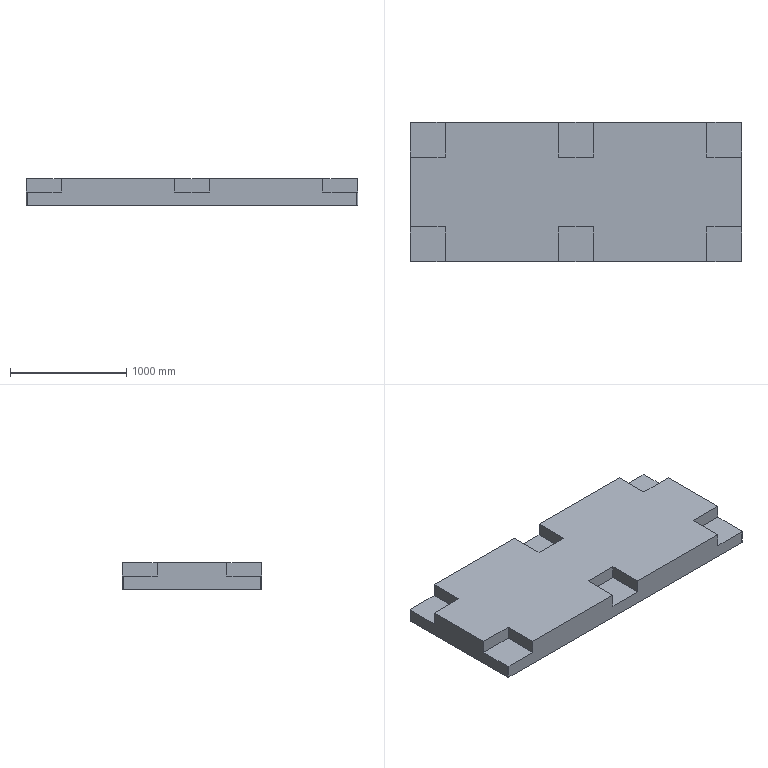Part | STEP file | 2850X1200X230MM-1.STEP | 1 solid | 30 faces | box 2850 x 1200 x 230 mm | volume 724490128 mm3 | plane 26 | cylinder 4 | commonest cylinder face diameters 20 x4
STEP:
#1=CARTESIAN_POINT('',(1425.,590.,115.));
#2=VERTEX_POINT('',#1);
#3=CARTESIAN_POINT('',(1415.,600.,115.));
#4=VERTEX_POINT('',#3);
#5=CARTESIAN_POINT('',(1415.,590.,115.));
#6=DIRECTION('',(0.,0.,1.));
#7=DIRECTION('',(1.,0.,0.));
#8=AXIS2_PLACEMENT_3D('',#5,#6,#7);
#9=CIRCLE('',#8,10.);
#10=EDGE_CURVE('',#2,#4,#9,.T.);
#11=ORIENTED_EDGE('',*,*,#10,.F.);
#12=CARTESIAN_POINT('',(1425.,590.,0.));
#13=VERTEX_POINT('',#12);
#14=CARTESIAN_POINT('',(1425.,590.,230.));
#15=DIRECTION('',(0.,0.,1.));
#16=VECTOR('',#15,1000.);
#17=LINE('',#14,#16);
#18=EDGE_CURVE('',#13,#2,#17,.T.);
#19=ORIENTED_EDGE('',*,*,#18,.F.);
#20=CARTESIAN_POINT('',(1415.,600.,0.));
#21=VERTEX_POINT('',#20);
#22=CARTESIAN_POINT('',(1415.,590.,0.));
#23=DIRECTION('',(0.,0.,-1.));
#24=DIRECTION('',(1.,0.,0.));
#25=AXIS2_PLACEMENT_3D('',#22,#23,#24);
#26=CIRCLE('',#25,10.);
#27=EDGE_CURVE('',#21,#13,#26,.T.);
#28=ORIENTED_EDGE('',*,*,#27,.F.);
#29=CARTESIAN_POINT('',(1415.,600.,230.));
#30=DIRECTION('',(0.,0.,-1.));
#31=VECTOR('',#30,1000.);
#32=LINE('',#29,#31);
#33=EDGE_CURVE('',#4,#21,#32,.T.);
#34=ORIENTED_EDGE('',*,*,#33,.F.);
#35=EDGE_LOOP('',(#11,#19,#28,#34));
#36=FACE_OUTER_BOUND('',#35,.T.);
#37=CARTESIAN_POINT('',(1415.,590.,230.));
#38=DIRECTION('',(0.,0.,-1.));
#39=DIRECTION('',(-1.,0.,0.));
#40=AXIS2_PLACEMENT_3D('',#37,#38,#39);
#41=CYLINDRICAL_SURFACE('',#40,10.);
#42=ADVANCED_FACE('',(#36),#41,.T.);
#43=CARTESIAN_POINT('',(-1415.,600.,115.));
#44=VERTEX_POINT('',#43);
#45=CARTESIAN_POINT('',(-1425.,590.,115.));
#46=VERTEX_POINT('',#45);
#47=CARTESIAN_POINT('',(-1415.,590.,115.));
#48=DIRECTION('',(0.,0.,1.));
#49=DIRECTION('',(1.,0.,0.));
#50=AXIS2_PLACEMENT_3D('',#47,#48,#49);
#51=CIRCLE('',#50,10.);
#52=EDGE_CURVE('',#44,#46,#51,.T.);
#53=ORIENTED_EDGE('',*,*,#52,.F.);
#54=CARTESIAN_POINT('',(-1415.,600.,0.));
#55=VERTEX_POINT('',#54);
#56=CARTESIAN_POINT('',(-1415.,600.,230.));
#57=DIRECTION('',(0.,0.,1.));
#58=VECTOR('',#57,1000.);
#59=LINE('',#56,#58);
#60=EDGE_CURVE('',#55,#44,#59,.T.);
#61=ORIENTED_EDGE('',*,*,#60,.F.);
#62=CARTESIAN_POINT('',(-1425.,590.,0.));
#63=VERTEX_POINT('',#62);
#64=CARTESIAN_POINT('',(-1415.,590.,0.));
#65=DIRECTION('',(0.,0.,-1.));
#66=DIRECTION('',(1.,0.,0.));
#67=AXIS2_PLACEMENT_3D('',#64,#65,#66);
#68=CIRCLE('',#67,10.);
#69=EDGE_CURVE('',#63,#55,#68,.T.);
#70=ORIENTED_EDGE('',*,*,#69,.F.);
#71=CARTESIAN_POINT('',(-1425.,590.,230.));
#72=DIRECTION('',(0.,0.,-1.));
#73=VECTOR('',#72,1000.);
#74=LINE('',#71,#73);
#75=EDGE_CURVE('',#46,#63,#74,.T.);
#76=ORIENTED_EDGE('',*,*,#75,.F.);
#77=EDGE_LOOP('',(#53,#61,#70,#76));
#78=FACE_OUTER_BOUND('',#77,.T.);
#79=CARTESIAN_POINT('',(-1415.,590.,230.));
#80=DIRECTION('',(0.,0.,-1.));
#81=DIRECTION('',(-1.,0.,0.));
#82=AXIS2_PLACEMENT_3D('',#79,#80,#81);
#83=CYLINDRICAL_SURFACE('',#82,10.);
#84=ADVANCED_FACE('',(#78),#83,.T.);
#85=CARTESIAN_POINT('',(-1425.,-590.,115.));
#86=VERTEX_POINT('',#85);
#87=CARTESIAN_POINT('',(-1415.,-600.,115.));
#88=VERTEX_POINT('',#87);
#89=CARTESIAN_POINT('',(-1415.,-590.,115.));
#90=DIRECTION('',(0.,0.,1.));
#91=DIRECTION('',(1.,0.,0.));
#92=AXIS2_PLACEMENT_3D('',#89,#90,#91);
#93=CIRCLE('',#92,10.);
#94=EDGE_CURVE('',#86,#88,#93,.T.);
#95=ORIENTED_EDGE('',*,*,#94,.F.);
#96=CARTESIAN_POINT('',(-1425.,-590.,0.));
#97=VERTEX_POINT('',#96);
#98=CARTESIAN_POINT('',(-1425.,-590.,230.));
#99=DIRECTION('',(0.,0.,1.));
#100=VECTOR('',#99,1000.);
#101=LINE('',#98,#100);
#102=EDGE_CURVE('',#97,#86,#101,.T.);
#103=ORIENTED_EDGE('',*,*,#102,.F.);
#104=CARTESIAN_POINT('',(-1415.,-600.,0.));
#105=VERTEX_POINT('',#104);
#106=CARTESIAN_POINT('',(-1415.,-590.,0.));
#107=DIRECTION('',(0.,0.,-1.));
#108=DIRECTION('',(1.,0.,0.));
#109=AXIS2_PLACEMENT_3D('',#106,#107,#108);
#110=CIRCLE('',#109,10.);
#111=EDGE_CURVE('',#105,#97,#110,.T.);
#112=ORIENTED_EDGE('',*,*,#111,.F.);
#113=CARTESIAN_POINT('',(-1415.,-600.,230.));
#114=DIRECTION('',(0.,0.,-1.));
#115=VECTOR('',#114,1000.);
#116=LINE('',#113,#115);
#117=EDGE_CURVE('',#88,#105,#116,.T.);
#118=ORIENTED_EDGE('',*,*,#117,.F.);
#119=EDGE_LOOP('',(#95,#103,#112,#118));
#120=FACE_OUTER_BOUND('',#119,.T.);
#121=CARTESIAN_POINT('',(-1415.,-590.,230.));
#122=DIRECTION('',(0.,0.,-1.));
#123=DIRECTION('',(-1.,0.,0.));
#124=AXIS2_PLACEMENT_3D('',#121,#122,#123);
#125=CYLINDRICAL_SURFACE('',#124,10.);
#126=ADVANCED_FACE('',(#120),#125,.T.);
#127=CARTESIAN_POINT('',(1415.,-600.,115.));
#128=VERTEX_POINT('',#127);
#129=CARTESIAN_POINT('',(1425.,-590.,115.));
#130=VERTEX_POINT('',#129);
#131=CARTESIAN_POINT('',(1415.,-590.,115.));
#132=DIRECTION('',(0.,0.,1.));
#133=DIRECTION('',(1.,0.,0.));
#134=AXIS2_PLACEMENT_3D('',#131,#132,#133);
#135=CIRCLE('',#134,10.);
#136=EDGE_CURVE('',#128,#130,#135,.T.);
#137=ORIENTED_EDGE('',*,*,#136,.F.);
#138=CARTESIAN_POINT('',(1415.,-600.,0.));
#139=VERTEX_POINT('',#138);
#140=CARTESIAN_POINT('',(1415.,-600.,230.));
#141=DIRECTION('',(0.,0.,1.));
#142=VECTOR('',#141,1000.);
#143=LINE('',#140,#142);
#144=EDGE_CURVE('',#139,#128,#143,.T.);
#145=ORIENTED_EDGE('',*,*,#144,.F.);
#146=CARTESIAN_POINT('',(1425.,-590.,0.));
#147=VERTEX_POINT('',#146);
#148=CARTESIAN_POINT('',(1415.,-590.,0.));
#149=DIRECTION('',(0.,0.,-1.));
#150=DIRECTION('',(1.,0.,0.));
#151=AXIS2_PLACEMENT_3D('',#148,#149,#150);
#152=CIRCLE('',#151,10.);
#153=EDGE_CURVE('',#147,#139,#152,.T.);
#154=ORIENTED_EDGE('',*,*,#153,.F.);
#155=CARTESIAN_POINT('',(1425.,-590.,230.));
#156=DIRECTION('',(0.,0.,-1.));
#157=VECTOR('',#156,1000.);
#158=LINE('',#155,#157);
#159=EDGE_CURVE('',#130,#147,#158,.T.);
#160=ORIENTED_EDGE('',*,*,#159,.F.);
#161=EDGE_LOOP('',(#137,#145,#154,#160));
#162=FACE_OUTER_BOUND('',#161,.T.);
#163=CARTESIAN_POINT('',(1415.,-590.,230.));
#164=DIRECTION('',(0.,0.,-1.));
#165=DIRECTION('',(-1.,0.,0.));
#166=AXIS2_PLACEMENT_3D('',#163,#164,#165);
#167=CYLINDRICAL_SURFACE('',#166,10.);
#168=ADVANCED_FACE('',(#162),#167,.T.);
#169=CARTESIAN_POINT('',(-1425.,-300.,115.));
#170=VERTEX_POINT('',#169);
#171=CARTESIAN_POINT('',(-1425.,-300.,115.));
#172=DIRECTION('',(0.,-1.,0.));
#173=VECTOR('',#172,1000.);
#174=LINE('',#171,#173);
#175=EDGE_CURVE('',#170,#86,#174,.T.);
#176=ORIENTED_EDGE('',*,*,#175,.T.);
#177=ORIENTED_EDGE('',*,*,#94,.T.);
#178=CARTESIAN_POINT('',(-1125.,-600.,115.));
#179=VERTEX_POINT('',#178);
#180=CARTESIAN_POINT('',(-1425.,-600.,115.));
#181=DIRECTION('',(1.,0.,0.));
#182=VECTOR('',#181,1000.);
#183=LINE('',#180,#182);
#184=EDGE_CURVE('',#88,#179,#183,.T.);
#185=ORIENTED_EDGE('',*,*,#184,.T.);
#186=CARTESIAN_POINT('',(-1125.,-300.,115.));
#187=VERTEX_POINT('',#186);
#188=CARTESIAN_POINT('',(-1125.,-300.,115.));
#189=DIRECTION('',(0.,1.,0.));
#190=VECTOR('',#189,1000.);
#191=LINE('',#188,#190);
#192=EDGE_CURVE('',#179,#187,#191,.T.);
#193=ORIENTED_EDGE('',*,*,#192,.T.);
#194=CARTESIAN_POINT('',(-1425.,-300.,115.));
#195=DIRECTION('',(-1.,0.,0.));
#196=VECTOR('',#195,1000.);
#197=LINE('',#194,#196);
#198=EDGE_CURVE('',#187,#170,#197,.T.);
#199=ORIENTED_EDGE('',*,*,#198,.T.);
#200=EDGE_LOOP('',(#176,#177,#185,#193,#199));
#201=FACE_OUTER_BOUND('',#200,.T.);
#202=CARTESIAN_POINT('',(0.,-900.,115.));
#203=DIRECTION('',(0.,0.,1.));
#204=DIRECTION('',(1.,0.,0.));
#205=AXIS2_PLACEMENT_3D('',#202,#203,#204);
#206=PLANE('',#205);
#207=ADVANCED_FACE('',(#201),#206,.T.);
#208=CARTESIAN_POINT('',(-1125.,-600.,230.));
#209=VERTEX_POINT('',#208);
#210=CARTESIAN_POINT('',(-1125.,-300.,230.));
#211=VERTEX_POINT('',#210);
#212=CARTESIAN_POINT('',(-1125.,-300.,230.));
#213=DIRECTION('',(0.,1.,0.));
#214=VECTOR('',#213,1000.);
#215=LINE('',#212,#214);
#216=EDGE_CURVE('',#209,#211,#215,.T.);
#217=ORIENTED_EDGE('',*,*,#216,.T.);
#218=CARTESIAN_POINT('',(-1125.,-300.,115.));
#219=DIRECTION('',(0.,0.,1.));
#220=VECTOR('',#219,1000.);
#221=LINE('',#218,#220);
#222=EDGE_CURVE('',#187,#211,#221,.T.);
#223=ORIENTED_EDGE('',*,*,#222,.F.);
#224=ORIENTED_EDGE('',*,*,#192,.F.);
#225=CARTESIAN_POINT('',(-1125.,-600.,115.));
#226=DIRECTION('',(0.,0.,1.));
#227=VECTOR('',#226,1000.);
#228=LINE('',#225,#227);
#229=EDGE_CURVE('',#179,#209,#228,.T.);
#230=ORIENTED_EDGE('',*,*,#229,.T.);
#231=EDGE_LOOP('',(#217,#223,#224,#230));
#232=FACE_OUTER_BOUND('',#231,.T.);
#233=CARTESIAN_POINT('',(-1125.,-300.,115.));
#234=DIRECTION('',(1.,0.,0.));
#235=DIRECTION('',(0.,1.,0.));
#236=AXIS2_PLACEMENT_3D('',#233,#234,#235);
#237=PLANE('',#236);
#238=ADVANCED_FACE('',(#232),#237,.F.);
#239=CARTESIAN_POINT('',(-1425.,-300.,230.));
#240=VERTEX_POINT('',#239);
#241=CARTESIAN_POINT('',(-1425.,-300.,230.));
#242=DIRECTION('',(-1.,0.,0.));
#243=VECTOR('',#242,1000.);
#244=LINE('',#241,#243);
#245=EDGE_CURVE('',#211,#240,#244,.T.);
#246=ORIENTED_EDGE('',*,*,#245,.T.);
#247=CARTESIAN_POINT('',(-1425.,-300.,115.));
#248=DIRECTION('',(0.,0.,1.));
#249=VECTOR('',#248,1000.);
#250=LINE('',#247,#249);
#251=EDGE_CURVE('',#170,#240,#250,.T.);
#252=ORIENTED_EDGE('',*,*,#251,.F.);
#253=ORIENTED_EDGE('',*,*,#198,.F.);
#254=ORIENTED_EDGE('',*,*,#222,.T.);
#255=EDGE_LOOP('',(#246,#252,#253,#254));
#256=FACE_OUTER_BOUND('',#255,.T.);
#257=CARTESIAN_POINT('',(-1425.,-300.,115.));
#258=DIRECTION('',(0.,1.,0.));
#259=DIRECTION('',(1.,0.,0.));
#260=AXIS2_PLACEMENT_3D('',#257,#258,#259);
#261=PLANE('',#260);
#262=ADVANCED_FACE('',(#256),#261,.F.);
#263=CARTESIAN_POINT('',(-150.,600.,115.));
#264=VERTEX_POINT('',#263);
#265=CARTESIAN_POINT('',(-150.,300.,115.));
#266=VERTEX_POINT('',#265);
#267=CARTESIAN_POINT('',(-150.,600.,115.));
#268=DIRECTION('',(0.,-1.,0.));
#269=VECTOR('',#268,1000.);
#270=LINE('',#267,#269);
#271=EDGE_CURVE('',#264,#266,#270,.T.);
#272=ORIENTED_EDGE('',*,*,#271,.T.);
#273=CARTESIAN_POINT('',(150.,300.,115.));
#274=VERTEX_POINT('',#273);
#275=CARTESIAN_POINT('',(-150.,300.,115.));
#276=DIRECTION('',(1.,0.,0.));
#277=VECTOR('',#276,1000.);
#278=LINE('',#275,#277);
#279=EDGE_CURVE('',#266,#274,#278,.T.);
#280=ORIENTED_EDGE('',*,*,#279,.T.);
#281=CARTESIAN_POINT('',(150.,600.,115.));
#282=VERTEX_POINT('',#281);
#283=CARTESIAN_POINT('',(150.,600.,115.));
#284=DIRECTION('',(0.,1.,0.));
#285=VECTOR('',#284,1000.);
#286=LINE('',#283,#285);
#287=EDGE_CURVE('',#274,#282,#286,.T.);
#288=ORIENTED_EDGE('',*,*,#287,.T.);
#289=CARTESIAN_POINT('',(-150.,600.,115.));
#290=DIRECTION('',(-1.,0.,0.));
#291=VECTOR('',#290,1000.);
#292=LINE('',#289,#291);
#293=EDGE_CURVE('',#282,#264,#292,.T.);
#294=ORIENTED_EDGE('',*,*,#293,.T.);
#295=EDGE_LOOP('',(#272,#280,#288,#294));
#296=FACE_OUTER_BOUND('',#295,.T.);
#297=CARTESIAN_POINT('',(1275.,0.,115.));
#298=DIRECTION('',(0.,0.,1.));
#299=DIRECTION('',(1.,0.,0.));
#300=AXIS2_PLACEMENT_3D('',#297,#298,#299);
#301=PLANE('',#300);
#302=ADVANCED_FACE('',(#296),#301,.T.);
#303=CARTESIAN_POINT('',(-150.,300.,230.));
#304=VERTEX_POINT('',#303);
#305=CARTESIAN_POINT('',(150.,300.,230.));
#306=VERTEX_POINT('',#305);
#307=CARTESIAN_POINT('',(-150.,300.,230.));
#308=DIRECTION('',(1.,0.,0.));
#309=VECTOR('',#308,1000.);
#310=LINE('',#307,#309);
#311=EDGE_CURVE('',#304,#306,#310,.T.);
#312=ORIENTED_EDGE('',*,*,#311,.T.);
#313=CARTESIAN_POINT('',(150.,300.,115.));
#314=DIRECTION('',(0.,0.,1.));
#315=VECTOR('',#314,1000.);
#316=LINE('',#313,#315);
#317=EDGE_CURVE('',#274,#306,#316,.T.);
#318=ORIENTED_EDGE('',*,*,#317,.F.);
#319=ORIENTED_EDGE('',*,*,#279,.F.);
#320=CARTESIAN_POINT('',(-150.,300.,115.));
#321=DIRECTION('',(0.,0.,1.));
#322=VECTOR('',#321,1000.);
#323=LINE('',#320,#322);
#324=EDGE_CURVE('',#266,#304,#323,.T.);
#325=ORIENTED_EDGE('',*,*,#324,.T.);
#326=EDGE_LOOP('',(#312,#318,#319,#325));
#327=FACE_OUTER_BOUND('',#326,.T.);
#328=CARTESIAN_POINT('',(-150.,300.,115.));
#329=DIRECTION('',(0.,-1.,0.));
#330=DIRECTION('',(0.,0.,-1.));
#331=AXIS2_PLACEMENT_3D('',#328,#329,#330);
#332=PLANE('',#331);
#333=ADVANCED_FACE('',(#327),#332,.F.);
#334=CARTESIAN_POINT('',(150.,600.,230.));
#335=VERTEX_POINT('',#334);
#336=CARTESIAN_POINT('',(150.,600.,230.));
#337=DIRECTION('',(0.,1.,0.));
#338=VECTOR('',#337,1000.);
#339=LINE('',#336,#338);
#340=EDGE_CURVE('',#306,#335,#339,.T.);
#341=ORIENTED_EDGE('',*,*,#340,.T.);
#342=CARTESIAN_POINT('',(150.,600.,115.));
#343=DIRECTION('',(0.,0.,1.));
#344=VECTOR('',#343,1000.);
#345=LINE('',#342,#344);
#346=EDGE_CURVE('',#282,#335,#345,.T.);
#347=ORIENTED_EDGE('',*,*,#346,.F.);
#348=ORIENTED_EDGE('',*,*,#287,.F.);
#349=ORIENTED_EDGE('',*,*,#317,.T.);
#350=EDGE_LOOP('',(#341,#347,#348,#349));
#351=FACE_OUTER_BOUND('',#350,.T.);
#352=CARTESIAN_POINT('',(150.,600.,115.));
#353=DIRECTION('',(1.,0.,0.));
#354=DIRECTION('',(0.,1.,0.));
#355=AXIS2_PLACEMENT_3D('',#352,#353,#354);
#356=PLANE('',#355);
#357=ADVANCED_FACE('',(#351),#356,.F.);
#358=CARTESIAN_POINT('',(-150.,600.,230.));
#359=VERTEX_POINT('',#358);
#360=CARTESIAN_POINT('',(-150.,600.,230.));
#361=DIRECTION('',(0.,-1.,0.));
#362=VECTOR('',#361,1000.);
#363=LINE('',#360,#362);
#364=EDGE_CURVE('',#359,#304,#363,.T.);
#365=ORIENTED_EDGE('',*,*,#364,.T.);
#366=ORIENTED_EDGE('',*,*,#324,.F.);
#367=ORIENTED_EDGE('',*,*,#271,.F.);
#368=CARTESIAN_POINT('',(-150.,600.,115.));
#369=DIRECTION('',(0.,0.,1.));
#370=VECTOR('',#369,1000.);
#371=LINE('',#368,#370);
#372=EDGE_CURVE('',#264,#359,#371,.T.);
#373=ORIENTED_EDGE('',*,*,#372,.T.);
#374=EDGE_LOOP('',(#365,#366,#367,#373));
#375=FACE_OUTER_BOUND('',#374,.T.);
#376=CARTESIAN_POINT('',(-150.,600.,115.));
#377=DIRECTION('',(-1.,0.,0.));
#378=DIRECTION('',(0.,0.,1.));
#379=AXIS2_PLACEMENT_3D('',#376,#377,#378);
#380=PLANE('',#379);
#381=ADVANCED_FACE('',(#375),#380,.F.);
#382=CARTESIAN_POINT('',(-150.,-300.,115.));
#383=VERTEX_POINT('',#382);
#384=CARTESIAN_POINT('',(-150.,-600.,115.));
#385=VERTEX_POINT('',#384);
#386=CARTESIAN_POINT('',(-150.,-300.,115.));
#387=DIRECTION('',(0.,-1.,0.));
#388=VECTOR('',#387,1000.);
#389=LINE('',#386,#388);
#390=EDGE_CURVE('',#383,#385,#389,.T.);
#391=ORIENTED_EDGE('',*,*,#390,.T.);
#392=CARTESIAN_POINT('',(150.,-600.,115.));
#393=VERTEX_POINT('',#392);
#394=CARTESIAN_POINT('',(-150.,-600.,115.));
#395=DIRECTION('',(1.,0.,0.));
#396=VECTOR('',#395,1000.);
#397=LINE('',#394,#396);
#398=EDGE_CURVE('',#385,#393,#397,.T.);
#399=ORIENTED_EDGE('',*,*,#398,.T.);
#400=CARTESIAN_POINT('',(150.,-300.,115.));
#401=VERTEX_POINT('',#400);
#402=CARTESIAN_POINT('',(150.,-300.,115.));
#403=DIRECTION('',(0.,1.,0.));
#404=VECTOR('',#403,1000.);
#405=LINE('',#402,#404);
#406=EDGE_CURVE('',#393,#401,#405,.T.);
#407=ORIENTED_EDGE('',*,*,#406,.T.);
#408=CARTESIAN_POINT('',(-150.,-300.,115.));
#409=DIRECTION('',(-1.,0.,0.));
#410=VECTOR('',#409,1000.);
#411=LINE('',#408,#410);
#412=EDGE_CURVE('',#401,#383,#411,.T.);
#413=ORIENTED_EDGE('',*,*,#412,.T.);
#414=EDGE_LOOP('',(#391,#399,#407,#413));
#415=FACE_OUTER_BOUND('',#414,.T.);
#416=CARTESIAN_POINT('',(1275.,-900.,115.));
#417=DIRECTION('',(0.,0.,1.));
#418=DIRECTION('',(1.,0.,0.));
#419=AXIS2_PLACEMENT_3D('',#416,#417,#418);
#420=PLANE('',#419);
#421=ADVANCED_FACE('',(#415),#420,.T.);
#422=CARTESIAN_POINT('',(150.,-600.,230.));
#423=VERTEX_POINT('',#422);
#424=CARTESIAN_POINT('',(150.,-300.,230.));
#425=VERTEX_POINT('',#424);
#426=CARTESIAN_POINT('',(150.,-300.,230.));
#427=DIRECTION('',(0.,1.,0.));
#428=VECTOR('',#427,1000.);
#429=LINE('',#426,#428);
#430=EDGE_CURVE('',#423,#425,#429,.T.);
#431=ORIENTED_EDGE('',*,*,#430,.T.);
#432=CARTESIAN_POINT('',(150.,-300.,115.));
#433=DIRECTION('',(0.,0.,1.));
#434=VECTOR('',#433,1000.);
#435=LINE('',#432,#434);
#436=EDGE_CURVE('',#401,#425,#435,.T.);
#437=ORIENTED_EDGE('',*,*,#436,.F.);
#438=ORIENTED_EDGE('',*,*,#406,.F.);
#439=CARTESIAN_POINT('',(150.,-600.,115.));
#440=DIRECTION('',(0.,0.,1.));
#441=VECTOR('',#440,1000.);
#442=LINE('',#439,#441);
#443=EDGE_CURVE('',#393,#423,#442,.T.);
#444=ORIENTED_EDGE('',*,*,#443,.T.);
#445=EDGE_LOOP('',(#431,#437,#438,#444));
#446=FACE_OUTER_BOUND('',#445,.T.);
#447=CARTESIAN_POINT('',(150.,-300.,115.));
#448=DIRECTION('',(1.,0.,0.));
#449=DIRECTION('',(0.,1.,0.));
#450=AXIS2_PLACEMENT_3D('',#447,#448,#449);
#451=PLANE('',#450);
#452=ADVANCED_FACE('',(#446),#451,.F.);
#453=CARTESIAN_POINT('',(-150.,-300.,230.));
#454=VERTEX_POINT('',#453);
#455=CARTESIAN_POINT('',(-150.,-300.,230.));
#456=DIRECTION('',(-1.,0.,0.));
#457=VECTOR('',#456,1000.);
#458=LINE('',#455,#457);
#459=EDGE_CURVE('',#425,#454,#458,.T.);
#460=ORIENTED_EDGE('',*,*,#459,.T.);
#461=CARTESIAN_POINT('',(-150.,-300.,115.));
#462=DIRECTION('',(0.,0.,1.));
#463=VECTOR('',#462,1000.);
#464=LINE('',#461,#463);
#465=EDGE_CURVE('',#383,#454,#464,.T.);
#466=ORIENTED_EDGE('',*,*,#465,.F.);
#467=ORIENTED_EDGE('',*,*,#412,.F.);
#468=ORIENTED_EDGE('',*,*,#436,.T.);
#469=EDGE_LOOP('',(#460,#466,#467,#468));
#470=FACE_OUTER_BOUND('',#469,.T.);
#471=CARTESIAN_POINT('',(-150.,-300.,115.));
#472=DIRECTION('',(0.,1.,0.));
#473=DIRECTION('',(1.,0.,0.));
#474=AXIS2_PLACEMENT_3D('',#471,#472,#473);
#475=PLANE('',#474);
#476=ADVANCED_FACE('',(#470),#475,.F.);
#477=CARTESIAN_POINT('',(-150.,-600.,230.));
#478=VERTEX_POINT('',#477);
#479=CARTESIAN_POINT('',(-150.,-300.,230.));
#480=DIRECTION('',(0.,-1.,0.));
#481=VECTOR('',#480,1000.);
#482=LINE('',#479,#481);
#483=EDGE_CURVE('',#454,#478,#482,.T.);
#484=ORIENTED_EDGE('',*,*,#483,.T.);
#485=CARTESIAN_POINT('',(-150.,-600.,115.));
#486=DIRECTION('',(0.,0.,1.));
#487=VECTOR('',#486,1000.);
#488=LINE('',#485,#487);
#489=EDGE_CURVE('',#385,#478,#488,.T.);
#490=ORIENTED_EDGE('',*,*,#489,.F.);
#491=ORIENTED_EDGE('',*,*,#390,.F.);
#492=ORIENTED_EDGE('',*,*,#465,.T.);
#493=EDGE_LOOP('',(#484,#490,#491,#492));
#494=FACE_OUTER_BOUND('',#493,.T.);
#495=CARTESIAN_POINT('',(-150.,-300.,115.));
#496=DIRECTION('',(-1.,0.,0.));
#497=DIRECTION('',(0.,0.,1.));
#498=AXIS2_PLACEMENT_3D('',#495,#496,#497);
#499=PLANE('',#498);
#500=ADVANCED_FACE('',(#494),#499,.F.);
#501=CARTESIAN_POINT('',(1425.,300.,115.));
#502=VERTEX_POINT('',#501);
#503=CARTESIAN_POINT('',(1425.,600.,115.));
#504=DIRECTION('',(0.,1.,0.));
#505=VECTOR('',#504,1000.);
#506=LINE('',#503,#505);
#507=EDGE_CURVE('',#502,#2,#506,.T.);
#508=ORIENTED_EDGE('',*,*,#507,.T.);
#509=ORIENTED_EDGE('',*,*,#10,.T.);
#510=CARTESIAN_POINT('',(1125.,600.,115.));
#511=VERTEX_POINT('',#510);
#512=CARTESIAN_POINT('',(1125.,600.,115.));
#513=DIRECTION('',(-1.,0.,0.));
#514=VECTOR('',#513,1000.);
#515=LINE('',#512,#514);
#516=EDGE_CURVE('',#4,#511,#515,.T.);
#517=ORIENTED_EDGE('',*,*,#516,.T.);
#518=CARTESIAN_POINT('',(1125.,300.,115.));
#519=VERTEX_POINT('',#518);
#520=CARTESIAN_POINT('',(1125.,600.,115.));
#521=DIRECTION('',(0.,-1.,0.));
#522=VECTOR('',#521,1000.);
#523=LINE('',#520,#522);
#524=EDGE_CURVE('',#511,#519,#523,.T.);
#525=ORIENTED_EDGE('',*,*,#524,.T.);
#526=CARTESIAN_POINT('',(1125.,300.,115.));
#527=DIRECTION('',(1.,0.,0.));
#528=VECTOR('',#527,1000.);
#529=LINE('',#526,#528);
#530=EDGE_CURVE('',#519,#502,#529,.T.);
#531=ORIENTED_EDGE('',*,*,#530,.T.);
#532=EDGE_LOOP('',(#508,#509,#517,#525,#531));
#533=FACE_OUTER_BOUND('',#532,.T.);
#534=CARTESIAN_POINT('',(2550.,0.,115.));
#535=DIRECTION('',(0.,0.,1.));
#536=DIRECTION('',(1.,0.,0.));
#537=AXIS2_PLACEMENT_3D('',#534,#535,#536);
#538=PLANE('',#537);
#539=ADVANCED_FACE('',(#533),#538,.T.);
#540=CARTESIAN_POINT('',(1125.,300.,230.));
#541=VERTEX_POINT('',#540);
#542=CARTESIAN_POINT('',(1425.,300.,230.));
#543=VERTEX_POINT('',#542);
#544=CARTESIAN_POINT('',(1125.,300.,230.));
#545=DIRECTION('',(1.,0.,0.));
#546=VECTOR('',#545,1000.);
#547=LINE('',#544,#546);
#548=EDGE_CURVE('',#541,#543,#547,.T.);
#549=ORIENTED_EDGE('',*,*,#548,.T.);
#550=CARTESIAN_POINT('',(1425.,300.,115.));
#551=DIRECTION('',(0.,0.,1.));
#552=VECTOR('',#551,1000.);
#553=LINE('',#550,#552);
#554=EDGE_CURVE('',#502,#543,#553,.T.);
#555=ORIENTED_EDGE('',*,*,#554,.F.);
#556=ORIENTED_EDGE('',*,*,#530,.F.);
#557=CARTESIAN_POINT('',(1125.,300.,115.));
#558=DIRECTION('',(0.,0.,1.));
#559=VECTOR('',#558,1000.);
#560=LINE('',#557,#559);
#561=EDGE_CURVE('',#519,#541,#560,.T.);
#562=ORIENTED_EDGE('',*,*,#561,.T.);
#563=EDGE_LOOP('',(#549,#555,#556,#562));
#564=FACE_OUTER_BOUND('',#563,.T.);
#565=CARTESIAN_POINT('',(1125.,300.,115.));
#566=DIRECTION('',(0.,-1.,0.));
#567=DIRECTION('',(0.,0.,-1.));
#568=AXIS2_PLACEMENT_3D('',#565,#566,#567);
#569=PLANE('',#568);
#570=ADVANCED_FACE('',(#564),#569,.F.);
#571=CARTESIAN_POINT('',(1125.,600.,230.));
#572=VERTEX_POINT('',#571);
#573=CARTESIAN_POINT('',(1125.,600.,230.));
#574=DIRECTION('',(0.,-1.,0.));
#575=VECTOR('',#574,1000.);
#576=LINE('',#573,#575);
#577=EDGE_CURVE('',#572,#541,#576,.T.);
#578=ORIENTED_EDGE('',*,*,#577,.T.);
#579=ORIENTED_EDGE('',*,*,#561,.F.);
#580=ORIENTED_EDGE('',*,*,#524,.F.);
#581=CARTESIAN_POINT('',(1125.,600.,115.));
#582=DIRECTION('',(0.,0.,1.));
#583=VECTOR('',#582,1000.);
#584=LINE('',#581,#583);
#585=EDGE_CURVE('',#511,#572,#584,.T.);
#586=ORIENTED_EDGE('',*,*,#585,.T.);
#587=EDGE_LOOP('',(#578,#579,#580,#586));
#588=FACE_OUTER_BOUND('',#587,.T.);
#589=CARTESIAN_POINT('',(1125.,600.,115.));
#590=DIRECTION('',(-1.,0.,0.));
#591=DIRECTION('',(0.,0.,1.));
#592=AXIS2_PLACEMENT_3D('',#589,#590,#591);
#593=PLANE('',#592);
#594=ADVANCED_FACE('',(#588),#593,.F.);
#595=CARTESIAN_POINT('',(1125.,-600.,115.));
#596=VERTEX_POINT('',#595);
#597=CARTESIAN_POINT('',(1125.,-600.,115.));
#598=DIRECTION('',(1.,0.,0.));
#599=VECTOR('',#598,1000.);
#600=LINE('',#597,#599);
#601=EDGE_CURVE('',#596,#128,#600,.T.);
#602=ORIENTED_EDGE('',*,*,#601,.T.);
#603=ORIENTED_EDGE('',*,*,#136,.T.);
#604=CARTESIAN_POINT('',(1425.,-300.,115.));
#605=VERTEX_POINT('',#604);
#606=CARTESIAN_POINT('',(1425.,-300.,115.));
#607=DIRECTION('',(0.,1.,0.));
#608=VECTOR('',#607,1000.);
#609=LINE('',#606,#608);
#610=EDGE_CURVE('',#130,#605,#609,.T.);
#611=ORIENTED_EDGE('',*,*,#610,.T.);
#612=CARTESIAN_POINT('',(1125.,-300.,115.));
#613=VERTEX_POINT('',#612);
#614=CARTESIAN_POINT('',(1125.,-300.,115.));
#615=DIRECTION('',(-1.,0.,0.));
#616=VECTOR('',#615,1000.);
#617=LINE('',#614,#616);
#618=EDGE_CURVE('',#605,#613,#617,.T.);
#619=ORIENTED_EDGE('',*,*,#618,.T.);
#620=CARTESIAN_POINT('',(1125.,-300.,115.));
#621=DIRECTION('',(0.,-1.,0.));
#622=VECTOR('',#621,1000.);
#623=LINE('',#620,#622);
#624=EDGE_CURVE('',#613,#596,#623,.T.);
#625=ORIENTED_EDGE('',*,*,#624,.T.);
#626=EDGE_LOOP('',(#602,#603,#611,#619,#625));
#627=FACE_OUTER_BOUND('',#626,.T.);
#628=CARTESIAN_POINT('',(2550.,-900.,115.));
#629=DIRECTION('',(0.,0.,1.));
#630=DIRECTION('',(1.,0.,0.));
#631=AXIS2_PLACEMENT_3D('',#628,#629,#630);
#632=PLANE('',#631);
#633=ADVANCED_FACE('',(#627),#632,.T.);
#634=CARTESIAN_POINT('',(1425.,-300.,230.));
#635=VERTEX_POINT('',#634);
#636=CARTESIAN_POINT('',(1125.,-300.,230.));
#637=VERTEX_POINT('',#636);
#638=CARTESIAN_POINT('',(1125.,-300.,230.));
#639=DIRECTION('',(-1.,0.,0.));
#640=VECTOR('',#639,1000.);
#641=LINE('',#638,#640);
#642=EDGE_CURVE('',#635,#637,#641,.T.);
#643=ORIENTED_EDGE('',*,*,#642,.T.);
#644=CARTESIAN_POINT('',(1125.,-300.,115.));
#645=DIRECTION('',(0.,0.,1.));
#646=VECTOR('',#645,1000.);
#647=LINE('',#644,#646);
#648=EDGE_CURVE('',#613,#637,#647,.T.);
#649=ORIENTED_EDGE('',*,*,#648,.F.);
#650=ORIENTED_EDGE('',*,*,#618,.F.);
#651=CARTESIAN_POINT('',(1425.,-300.,115.));
#652=DIRECTION('',(0.,0.,1.));
#653=VECTOR('',#652,1000.);
#654=LINE('',#651,#653);
#655=EDGE_CURVE('',#605,#635,#654,.T.);
#656=ORIENTED_EDGE('',*,*,#655,.T.);
#657=EDGE_LOOP('',(#643,#649,#650,#656));
#658=FACE_OUTER_BOUND('',#657,.T.);
#659=CARTESIAN_POINT('',(1125.,-300.,115.));
#660=DIRECTION('',(0.,1.,0.));
#661=DIRECTION('',(1.,0.,0.));
#662=AXIS2_PLACEMENT_3D('',#659,#660,#661);
#663=PLANE('',#662);
#664=ADVANCED_FACE('',(#658),#663,.F.);
#665=CARTESIAN_POINT('',(1125.,-600.,230.));
#666=VERTEX_POINT('',#665);
#667=CARTESIAN_POINT('',(1125.,-300.,230.));
#668=DIRECTION('',(0.,-1.,0.));
#669=VECTOR('',#668,1000.);
#670=LINE('',#667,#669);
#671=EDGE_CURVE('',#637,#666,#670,.T.);
#672=ORIENTED_EDGE('',*,*,#671,.T.);
#673=CARTESIAN_POINT('',(1125.,-600.,115.));
#674=DIRECTION('',(0.,0.,1.));
#675=VECTOR('',#674,1000.);
#676=LINE('',#673,#675);
#677=EDGE_CURVE('',#596,#666,#676,.T.);
#678=ORIENTED_EDGE('',*,*,#677,.F.);
#679=ORIENTED_EDGE('',*,*,#624,.F.);
#680=ORIENTED_EDGE('',*,*,#648,.T.);
#681=EDGE_LOOP('',(#672,#678,#679,#680));
#682=FACE_OUTER_BOUND('',#681,.T.);
#683=CARTESIAN_POINT('',(1125.,-300.,115.));
#684=DIRECTION('',(-1.,0.,0.));
#685=DIRECTION('',(0.,0.,1.));
#686=AXIS2_PLACEMENT_3D('',#683,#684,#685);
#687=PLANE('',#686);
#688=ADVANCED_FACE('',(#682),#687,.F.);
#689=CARTESIAN_POINT('',(-1125.,600.,115.));
#690=VERTEX_POINT('',#689);
#691=CARTESIAN_POINT('',(-1425.,600.,115.));
#692=DIRECTION('',(-1.,0.,0.));
#693=VECTOR('',#692,1000.);
#694=LINE('',#691,#693);
#695=EDGE_CURVE('',#690,#44,#694,.T.);
#696=ORIENTED_EDGE('',*,*,#695,.T.);
#697=ORIENTED_EDGE('',*,*,#52,.T.);
#698=CARTESIAN_POINT('',(-1425.,300.,115.));
#699=VERTEX_POINT('',#698);
#700=CARTESIAN_POINT('',(-1425.,600.,115.));
#701=DIRECTION('',(0.,-1.,0.));
#702=VECTOR('',#701,1000.);
#703=LINE('',#700,#702);
#704=EDGE_CURVE('',#46,#699,#703,.T.);
#705=ORIENTED_EDGE('',*,*,#704,.T.);
#706=CARTESIAN_POINT('',(-1125.,300.,115.));
#707=VERTEX_POINT('',#706);
#708=CARTESIAN_POINT('',(-1425.,300.,115.));
#709=DIRECTION('',(1.,0.,0.));
#710=VECTOR('',#709,1000.);
#711=LINE('',#708,#710);
#712=EDGE_CURVE('',#699,#707,#711,.T.);
#713=ORIENTED_EDGE('',*,*,#712,.T.);
#714=CARTESIAN_POINT('',(-1125.,600.,115.));
#715=DIRECTION('',(0.,1.,0.));
#716=VECTOR('',#715,1000.);
#717=LINE('',#714,#716);
#718=EDGE_CURVE('',#707,#690,#717,.T.);
#719=ORIENTED_EDGE('',*,*,#718,.T.);
#720=EDGE_LOOP('',(#696,#697,#705,#713,#719));
#721=FACE_OUTER_BOUND('',#720,.T.);
#722=CARTESIAN_POINT('',(0.,0.,115.));
#723=DIRECTION('',(0.,0.,1.));
#724=DIRECTION('',(1.,0.,0.));
#725=AXIS2_PLACEMENT_3D('',#722,#723,#724);
#726=PLANE('',#725);
#727=ADVANCED_FACE('',(#721),#726,.T.);
#728=CARTESIAN_POINT('',(-1425.,300.,230.));
#729=VERTEX_POINT('',#728);
#730=CARTESIAN_POINT('',(-1125.,300.,230.));
#731=VERTEX_POINT('',#730);
#732=CARTESIAN_POINT('',(-1425.,300.,230.));
#733=DIRECTION('',(1.,0.,0.));
#734=VECTOR('',#733,1000.);
#735=LINE('',#732,#734);
#736=EDGE_CURVE('',#729,#731,#735,.T.);
#737=ORIENTED_EDGE('',*,*,#736,.T.);
#738=CARTESIAN_POINT('',(-1125.,300.,115.));
#739=DIRECTION('',(0.,0.,1.));
#740=VECTOR('',#739,1000.);
#741=LINE('',#738,#740);
#742=EDGE_CURVE('',#707,#731,#741,.T.);
#743=ORIENTED_EDGE('',*,*,#742,.F.);
#744=ORIENTED_EDGE('',*,*,#712,.F.);
#745=CARTESIAN_POINT('',(-1425.,300.,115.));
#746=DIRECTION('',(0.,0.,1.));
#747=VECTOR('',#746,1000.);
#748=LINE('',#745,#747);
#749=EDGE_CURVE('',#699,#729,#748,.T.);
#750=ORIENTED_EDGE('',*,*,#749,.T.);
#751=EDGE_LOOP('',(#737,#743,#744,#750));
#752=FACE_OUTER_BOUND('',#751,.T.);
#753=CARTESIAN_POINT('',(-1425.,300.,115.));
#754=DIRECTION('',(0.,-1.,0.));
#755=DIRECTION('',(0.,0.,-1.));
#756=AXIS2_PLACEMENT_3D('',#753,#754,#755);
#757=PLANE('',#756);
#758=ADVANCED_FACE('',(#752),#757,.F.);
#759=CARTESIAN_POINT('',(-1125.,600.,230.));
#760=VERTEX_POINT('',#759);
#761=CARTESIAN_POINT('',(-1125.,600.,230.));
#762=DIRECTION('',(0.,1.,0.));
#763=VECTOR('',#762,1000.);
#764=LINE('',#761,#763);
#765=EDGE_CURVE('',#731,#760,#764,.T.);
#766=ORIENTED_EDGE('',*,*,#765,.T.);
#767=CARTESIAN_POINT('',(-1125.,600.,115.));
#768=DIRECTION('',(0.,0.,1.));
#769=VECTOR('',#768,1000.);
#770=LINE('',#767,#769);
#771=EDGE_CURVE('',#690,#760,#770,.T.);
#772=ORIENTED_EDGE('',*,*,#771,.F.);
#773=ORIENTED_EDGE('',*,*,#718,.F.);
#774=ORIENTED_EDGE('',*,*,#742,.T.);
#775=EDGE_LOOP('',(#766,#772,#773,#774));
#776=FACE_OUTER_BOUND('',#775,.T.);
#777=CARTESIAN_POINT('',(-1125.,600.,115.));
#778=DIRECTION('',(1.,0.,0.));
#779=DIRECTION('',(0.,1.,0.));
#780=AXIS2_PLACEMENT_3D('',#777,#778,#779);
#781=PLANE('',#780);
#782=ADVANCED_FACE('',(#776),#781,.F.);
#783=CARTESIAN_POINT('',(1425.,600.,0.));
#784=DIRECTION('',(0.,1.,0.));
#785=VECTOR('',#784,1000.);
#786=LINE('',#783,#785);
#787=EDGE_CURVE('',#147,#13,#786,.T.);
#788=ORIENTED_EDGE('',*,*,#787,.F.);
#789=ORIENTED_EDGE('',*,*,#153,.T.);
#790=CARTESIAN_POINT('',(-1425.,-600.,0.));
#791=DIRECTION('',(1.,0.,0.));
#792=VECTOR('',#791,1000.);
#793=LINE('',#790,#792);
#794=EDGE_CURVE('',#105,#139,#793,.T.);
#795=ORIENTED_EDGE('',*,*,#794,.F.);
#796=ORIENTED_EDGE('',*,*,#111,.T.);
#797=CARTESIAN_POINT('',(-1425.,600.,0.));
#798=DIRECTION('',(0.,-1.,0.));
#799=VECTOR('',#798,1000.);
#800=LINE('',#797,#799);
#801=EDGE_CURVE('',#63,#97,#800,.T.);
#802=ORIENTED_EDGE('',*,*,#801,.F.);
#803=ORIENTED_EDGE('',*,*,#69,.T.);
#804=CARTESIAN_POINT('',(-1425.,600.,0.));
#805=DIRECTION('',(-1.,0.,0.));
#806=VECTOR('',#805,1000.);
#807=LINE('',#804,#806);
#808=EDGE_CURVE('',#21,#55,#807,.T.);
#809=ORIENTED_EDGE('',*,*,#808,.F.);
#810=ORIENTED_EDGE('',*,*,#27,.T.);
#811=EDGE_LOOP('',(#788,#789,#795,#796,#802,#803,#809,#810));
#812=FACE_OUTER_BOUND('',#811,.T.);
#813=CARTESIAN_POINT('',(0.,0.,0.));
#814=DIRECTION('',(0.,0.,1.));
#815=DIRECTION('',(1.,0.,0.));
#816=AXIS2_PLACEMENT_3D('',#813,#814,#815);
#817=PLANE('',#816);
#818=ADVANCED_FACE('',(#812),#817,.F.);
#819=ORIENTED_EDGE('',*,*,#245,.F.);
#820=ORIENTED_EDGE('',*,*,#216,.F.);
#821=CARTESIAN_POINT('',(-1425.,-600.,230.));
#822=DIRECTION('',(1.,0.,0.));
#823=VECTOR('',#822,1000.);
#824=LINE('',#821,#823);
#825=EDGE_CURVE('',#209,#478,#824,.T.);
#826=ORIENTED_EDGE('',*,*,#825,.T.);
#827=ORIENTED_EDGE('',*,*,#483,.F.);
#828=ORIENTED_EDGE('',*,*,#459,.F.);
#829=ORIENTED_EDGE('',*,*,#430,.F.);
#830=CARTESIAN_POINT('',(-1425.,-600.,230.));
#831=DIRECTION('',(1.,0.,0.));
#832=VECTOR('',#831,1000.);
#833=LINE('',#830,#832);
#834=EDGE_CURVE('',#423,#666,#833,.T.);
#835=ORIENTED_EDGE('',*,*,#834,.T.);
#836=ORIENTED_EDGE('',*,*,#671,.F.);
#837=ORIENTED_EDGE('',*,*,#642,.F.);
#838=CARTESIAN_POINT('',(1425.,600.,230.));
#839=DIRECTION('',(0.,1.,0.));
#840=VECTOR('',#839,1000.);
#841=LINE('',#838,#840);
#842=EDGE_CURVE('',#635,#543,#841,.T.);
#843=ORIENTED_EDGE('',*,*,#842,.T.);
#844=ORIENTED_EDGE('',*,*,#548,.F.);
#845=ORIENTED_EDGE('',*,*,#577,.F.);
#846=CARTESIAN_POINT('',(-1425.,600.,230.));
#847=DIRECTION('',(-1.,0.,0.));
#848=VECTOR('',#847,1000.);
#849=LINE('',#846,#848);
#850=EDGE_CURVE('',#572,#335,#849,.T.);
#851=ORIENTED_EDGE('',*,*,#850,.T.);
#852=ORIENTED_EDGE('',*,*,#340,.F.);
#853=ORIENTED_EDGE('',*,*,#311,.F.);
#854=ORIENTED_EDGE('',*,*,#364,.F.);
#855=CARTESIAN_POINT('',(-1425.,600.,230.));
#856=DIRECTION('',(-1.,0.,0.));
#857=VECTOR('',#856,1000.);
#858=LINE('',#855,#857);
#859=EDGE_CURVE('',#359,#760,#858,.T.);
#860=ORIENTED_EDGE('',*,*,#859,.T.);
#861=ORIENTED_EDGE('',*,*,#765,.F.);
#862=ORIENTED_EDGE('',*,*,#736,.F.);
#863=CARTESIAN_POINT('',(-1425.,600.,230.));
#864=DIRECTION('',(0.,-1.,0.));
#865=VECTOR('',#864,1000.);
#866=LINE('',#863,#865);
#867=EDGE_CURVE('',#729,#240,#866,.T.);
#868=ORIENTED_EDGE('',*,*,#867,.T.);
#869=EDGE_LOOP('',(#819,#820,#826,#827,#828,#829,#835,#836,#837,#843,#844,#845,#851,#852,#853,#854,#860,#861,#862,#868));
#870=FACE_OUTER_BOUND('',#869,.T.);
#871=CARTESIAN_POINT('',(0.,0.,230.));
#872=DIRECTION('',(0.,0.,1.));
#873=DIRECTION('',(1.,0.,0.));
#874=AXIS2_PLACEMENT_3D('',#871,#872,#873);
#875=PLANE('',#874);
#876=ADVANCED_FACE('',(#870),#875,.T.);
#877=ORIENTED_EDGE('',*,*,#794,.T.);
#878=ORIENTED_EDGE('',*,*,#144,.T.);
#879=ORIENTED_EDGE('',*,*,#601,.F.);
#880=ORIENTED_EDGE('',*,*,#677,.T.);
#881=ORIENTED_EDGE('',*,*,#834,.F.);
#882=ORIENTED_EDGE('',*,*,#443,.F.);
#883=ORIENTED_EDGE('',*,*,#398,.F.);
#884=ORIENTED_EDGE('',*,*,#489,.T.);
#885=ORIENTED_EDGE('',*,*,#825,.F.);
#886=ORIENTED_EDGE('',*,*,#229,.F.);
#887=ORIENTED_EDGE('',*,*,#184,.F.);
#888=ORIENTED_EDGE('',*,*,#117,.T.);
#889=EDGE_LOOP('',(#877,#878,#879,#880,#881,#882,#883,#884,#885,#886,#887,#888));
#890=FACE_OUTER_BOUND('',#889,.T.);
#891=CARTESIAN_POINT('',(-1425.,-600.,230.));
#892=DIRECTION('',(0.,1.,0.));
#893=DIRECTION('',(1.,0.,0.));
#894=AXIS2_PLACEMENT_3D('',#891,#892,#893);
#895=PLANE('',#894);
#896=ADVANCED_FACE('',(#890),#895,.F.);
#897=ORIENTED_EDGE('',*,*,#801,.T.);
#898=ORIENTED_EDGE('',*,*,#102,.T.);
#899=ORIENTED_EDGE('',*,*,#175,.F.);
#900=ORIENTED_EDGE('',*,*,#251,.T.);
#901=ORIENTED_EDGE('',*,*,#867,.F.);
#902=ORIENTED_EDGE('',*,*,#749,.F.);
#903=ORIENTED_EDGE('',*,*,#704,.F.);
#904=ORIENTED_EDGE('',*,*,#75,.T.);
#905=EDGE_LOOP('',(#897,#898,#899,#900,#901,#902,#903,#904));
#906=FACE_OUTER_BOUND('',#905,.T.);
#907=CARTESIAN_POINT('',(-1425.,600.,230.));
#908=DIRECTION('',(1.,0.,0.));
#909=DIRECTION('',(0.,1.,0.));
#910=AXIS2_PLACEMENT_3D('',#907,#908,#909);
#911=PLANE('',#910);
#912=ADVANCED_FACE('',(#906),#911,.F.);
#913=ORIENTED_EDGE('',*,*,#808,.T.);
#914=ORIENTED_EDGE('',*,*,#60,.T.);
#915=ORIENTED_EDGE('',*,*,#695,.F.);
#916=ORIENTED_EDGE('',*,*,#771,.T.);
#917=ORIENTED_EDGE('',*,*,#859,.F.);
#918=ORIENTED_EDGE('',*,*,#372,.F.);
#919=ORIENTED_EDGE('',*,*,#293,.F.);
#920=ORIENTED_EDGE('',*,*,#346,.T.);
#921=ORIENTED_EDGE('',*,*,#850,.F.);
#922=ORIENTED_EDGE('',*,*,#585,.F.);
#923=ORIENTED_EDGE('',*,*,#516,.F.);
#924=ORIENTED_EDGE('',*,*,#33,.T.);
#925=EDGE_LOOP('',(#913,#914,#915,#916,#917,#918,#919,#920,#921,#922,#923,#924));
#926=FACE_OUTER_BOUND('',#925,.T.);
#927=CARTESIAN_POINT('',(-1425.,600.,230.));
#928=DIRECTION('',(0.,-1.,0.));
#929=DIRECTION('',(0.,0.,-1.));
#930=AXIS2_PLACEMENT_3D('',#927,#928,#929);
#931=PLANE('',#930);
#932=ADVANCED_FACE('',(#926),#931,.F.);
#933=ORIENTED_EDGE('',*,*,#610,.F.);
#934=ORIENTED_EDGE('',*,*,#159,.T.);
#935=ORIENTED_EDGE('',*,*,#787,.T.);
#936=ORIENTED_EDGE('',*,*,#18,.T.);
#937=ORIENTED_EDGE('',*,*,#507,.F.);
#938=ORIENTED_EDGE('',*,*,#554,.T.);
#939=ORIENTED_EDGE('',*,*,#842,.F.);
#940=ORIENTED_EDGE('',*,*,#655,.F.);
#941=EDGE_LOOP('',(#933,#934,#935,#936,#937,#938,#939,#940));
#942=FACE_OUTER_BOUND('',#941,.T.);
#943=CARTESIAN_POINT('',(1425.,600.,230.));
#944=DIRECTION('',(-1.,0.,0.));
#945=DIRECTION('',(0.,0.,1.));
#946=AXIS2_PLACEMENT_3D('',#943,#944,#945);
#947=PLANE('',#946);
#948=ADVANCED_FACE('',(#942),#947,.F.);
#949=CLOSED_SHELL('',(#42,#84,#126,#168,#207,#238,#262,#302,#333,#357,#381,#421,#452,#476,#500,#539,#570,#594,#633,#664,#688,#727,#758,#782,#818,#876,#896,#912,#932,#948));
#950=MANIFOLD_SOLID_BREP('',#949);
#951=CARTESIAN_POINT('',(0.,0.,0.));
#952=DIRECTION('',(0.,0.,1.));
#953=DIRECTION('',(1.,0.,0.));
#954=AXIS2_PLACEMENT_3D('',#951,#952,#953);
#955=(LENGTH_UNIT()NAMED_UNIT(*)SI_UNIT(.MILLI.,.METRE.));
#956=UNCERTAINTY_MEASURE_WITH_UNIT(LENGTH_MEASURE(0.00001),#955,'','');
#957=(NAMED_UNIT(*)PLANE_ANGLE_UNIT()SI_UNIT($,.RADIAN.));
#958=(NAMED_UNIT(*)SI_UNIT($,.STERADIAN.)SOLID_ANGLE_UNIT());
#959=(GEOMETRIC_REPRESENTATION_CONTEXT(3)GLOBAL_UNCERTAINTY_ASSIGNED_CONTEXT((#956))GLOBAL_UNIT_ASSIGNED_CONTEXT((#955,#957,#958))REPRESENTATION_CONTEXT('',''));
#960=ADVANCED_BREP_SHAPE_REPRESENTATION('',(#950,#954),#959);